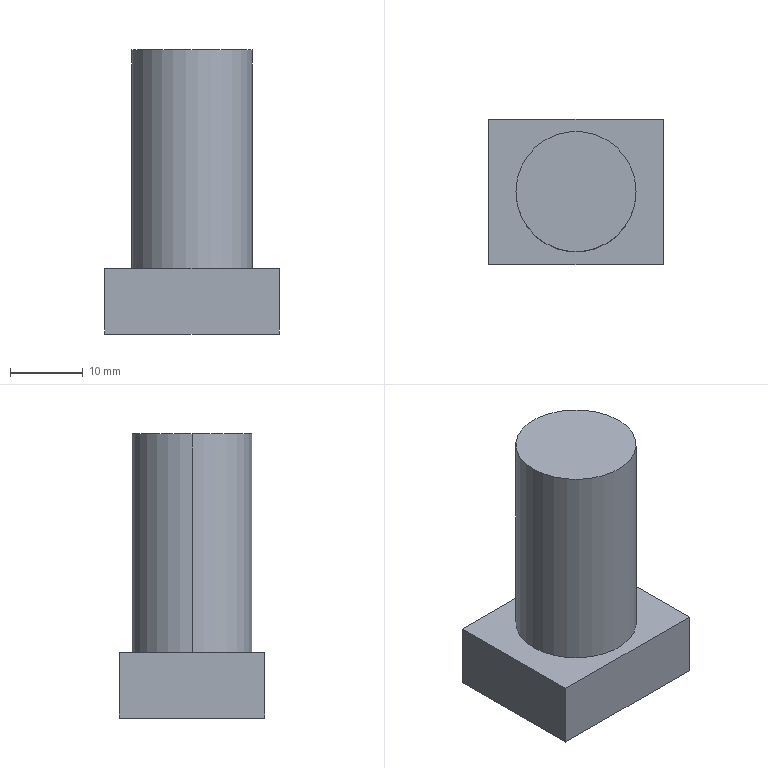Part | STEP file | Button | 1 solid | 9 faces | box 24 x 20 x 39 mm | volume 10735 mm3 | plane 7 | cylinder 2 | commonest cylinder face diameters 16.5 x2
STEP:
#1=CARTESIAN_POINT('',(0.,0.,0.));
#2=DIRECTION('',(0.,0.,1.));
#3=DIRECTION('',(1.,0.,0.));
#4=AXIS2_PLACEMENT_3D('',#1,#2,#3);
#5=CARTESIAN_POINT('',(-8.25,0.,39.));
#6=VERTEX_POINT('',#5);
#7=CARTESIAN_POINT('',(8.25,0.,39.));
#8=VERTEX_POINT('',#7);
#9=CARTESIAN_POINT('',(0.,0.,39.));
#10=DIRECTION('',(0.,0.,-1.));
#11=DIRECTION('',(-1.,0.,0.));
#12=AXIS2_PLACEMENT_3D('',#9,#10,#11);
#13=CIRCLE('',#12,8.25);
#14=CARTESIAN_POINT('',(0.,0.,39.));
#15=DIRECTION('',(0.,0.,-1.));
#16=DIRECTION('',(-1.,0.,0.));
#17=AXIS2_PLACEMENT_3D('',#14,#15,#16);
#18=CYLINDRICAL_SURFACE('',#17,8.25);
#19=CARTESIAN_POINT('',(0.,0.));
#20=DIRECTION('',(1.,0.));
#21=VECTOR('',#20,1.);
#22=LINE('',#19,#21);
#23=(GEOMETRIC_REPRESENTATION_CONTEXT(2)PARAMETRIC_REPRESENTATION_CONTEXT()REPRESENTATION_CONTEXT('',''));
#24=DEFINITIONAL_REPRESENTATION('',(#22),#23);
#25=PCURVE('',#18,#24);
#26=CARTESIAN_POINT('',(0.,0.,39.));
#27=DIRECTION('',(0.,0.,1.));
#28=DIRECTION('',(1.,0.,0.));
#29=AXIS2_PLACEMENT_3D('',#26,#27,#28);
#30=PLANE('',#29);
#31=CARTESIAN_POINT('',(-8.25,0.));
#32=CARTESIAN_POINT('',(-8.25,14.289));
#33=CARTESIAN_POINT('',(4.125,7.145));
#34=CARTESIAN_POINT('',(16.5,0.));
#35=CARTESIAN_POINT('',(4.125,-7.145));
#36=CARTESIAN_POINT('',(-8.25,-14.289));
#37=CARTESIAN_POINT('',(-8.25,0.));
#38=(BOUNDED_CURVE()B_SPLINE_CURVE(2,(#31,#32,#33,#34,#35,#36,#37),.UNSPECIFIED.,.T.,.F.)B_SPLINE_CURVE_WITH_KNOTS((1,2,2,2,2,1),(-2.094,0.,2.094,4.189,6.283,8.378),.UNSPECIFIED.)CURVE()GEOMETRIC_REPRESENTATION_ITEM()RATIONAL_B_SPLINE_CURVE((1.,0.5,1.,0.5,1.,0.5,1.))REPRESENTATION_ITEM(''));
#39=(GEOMETRIC_REPRESENTATION_CONTEXT(2)PARAMETRIC_REPRESENTATION_CONTEXT()REPRESENTATION_CONTEXT('',''));
#40=DEFINITIONAL_REPRESENTATION('',(#38),#39);
#41=PCURVE('',#30,#40);
#42=SURFACE_CURVE('',#13,(#25,#41),.PCURVE_S1.);
#43=EDGE_CURVE('',#6,#8,#42,.T.);
#44=ORIENTED_EDGE('',*,*,#43,.T.);
#45=CARTESIAN_POINT('',(8.25,0.,9.));
#46=VERTEX_POINT('',#45);
#47=CARTESIAN_POINT('',(8.25,0.,39.));
#48=DIRECTION('',(0.,0.,-1.));
#49=VECTOR('',#48,1.);
#50=LINE('',#47,#49);
#51=CARTESIAN_POINT('',(3.142,0.));
#52=DIRECTION('',(0.,1.));
#53=VECTOR('',#52,1.);
#54=LINE('',#51,#53);
#55=(GEOMETRIC_REPRESENTATION_CONTEXT(2)PARAMETRIC_REPRESENTATION_CONTEXT()REPRESENTATION_CONTEXT('',''));
#56=DEFINITIONAL_REPRESENTATION('',(#54),#55);
#57=PCURVE('',#18,#56);
#58=CARTESIAN_POINT('',(0.,0.,39.));
#59=DIRECTION('',(0.,0.,-1.));
#60=DIRECTION('',(-1.,0.,0.));
#61=AXIS2_PLACEMENT_3D('',#58,#59,#60);
#62=CYLINDRICAL_SURFACE('',#61,8.25);
#63=CARTESIAN_POINT('',(3.142,0.));
#64=DIRECTION('',(0.,1.));
#65=VECTOR('',#64,1.);
#66=LINE('',#63,#65);
#67=(GEOMETRIC_REPRESENTATION_CONTEXT(2)PARAMETRIC_REPRESENTATION_CONTEXT()REPRESENTATION_CONTEXT('',''));
#68=DEFINITIONAL_REPRESENTATION('',(#66),#67);
#69=PCURVE('',#62,#68);
#70=SURFACE_CURVE('',#50,(#57,#69),.PCURVE_S1.);
#71=EDGE_CURVE('',#8,#46,#70,.T.);
#72=ORIENTED_EDGE('',*,*,#71,.T.);
#73=CARTESIAN_POINT('',(-8.25,0.,9.));
#74=VERTEX_POINT('',#73);
#75=CARTESIAN_POINT('',(0.,0.,9.));
#76=DIRECTION('',(0.,0.,1.));
#77=DIRECTION('',(-1.,0.,0.));
#78=AXIS2_PLACEMENT_3D('',#75,#76,#77);
#79=CIRCLE('',#78,8.25);
#80=CARTESIAN_POINT('',(6.283,30.));
#81=DIRECTION('',(-1.,0.));
#82=VECTOR('',#81,1.);
#83=LINE('',#80,#82);
#84=(GEOMETRIC_REPRESENTATION_CONTEXT(2)PARAMETRIC_REPRESENTATION_CONTEXT()REPRESENTATION_CONTEXT('',''));
#85=DEFINITIONAL_REPRESENTATION('',(#83),#84);
#86=PCURVE('',#18,#85);
#87=CARTESIAN_POINT('',(-12.,-10.,9.));
#88=DIRECTION('',(0.,0.,1.));
#89=DIRECTION('',(1.,0.,0.));
#90=AXIS2_PLACEMENT_3D('',#87,#88,#89);
#91=PLANE('',#90);
#92=CARTESIAN_POINT('',(12.,10.));
#93=DIRECTION('',(-1.,0.));
#94=AXIS2_PLACEMENT_2D('',#92,#93);
#95=CIRCLE('',#94,8.25);
#96=(GEOMETRIC_REPRESENTATION_CONTEXT(2)PARAMETRIC_REPRESENTATION_CONTEXT()REPRESENTATION_CONTEXT('',''));
#97=DEFINITIONAL_REPRESENTATION('',(#95),#96);
#98=PCURVE('',#91,#97);
#99=SURFACE_CURVE('',#79,(#86,#98),.PCURVE_S1.);
#100=EDGE_CURVE('',#46,#74,#99,.T.);
#101=ORIENTED_EDGE('',*,*,#100,.T.);
#102=CARTESIAN_POINT('',(-8.25,0.,39.));
#103=DIRECTION('',(0.,0.,-1.));
#104=VECTOR('',#103,1.);
#105=LINE('',#102,#104);
#106=CARTESIAN_POINT('',(0.,0.));
#107=DIRECTION('',(0.,1.));
#108=VECTOR('',#107,1.);
#109=LINE('',#106,#108);
#110=(GEOMETRIC_REPRESENTATION_CONTEXT(2)PARAMETRIC_REPRESENTATION_CONTEXT()REPRESENTATION_CONTEXT('',''));
#111=DEFINITIONAL_REPRESENTATION('',(#109),#110);
#112=PCURVE('',#18,#111);
#113=CARTESIAN_POINT('',(6.283,0.));
#114=DIRECTION('',(0.,1.));
#115=VECTOR('',#114,1.);
#116=LINE('',#113,#115);
#117=(GEOMETRIC_REPRESENTATION_CONTEXT(2)PARAMETRIC_REPRESENTATION_CONTEXT()REPRESENTATION_CONTEXT('',''));
#118=DEFINITIONAL_REPRESENTATION('',(#116),#117);
#119=PCURVE('',#62,#118);
#120=SURFACE_CURVE('',#105,(#112,#119),.PCURVE_S1.);
#121=EDGE_CURVE('',#6,#74,#120,.T.);
#122=ORIENTED_EDGE('',*,*,#121,.F.);
#123=EDGE_LOOP('',(#44,#72,#101,#122));
#124=FACE_BOUND('',#123,.T.);
#125=ADVANCED_FACE('',(#124),#18,.T.);
#126=ORIENTED_EDGE('',*,*,#71,.F.);
#127=CARTESIAN_POINT('',(0.,0.,39.));
#128=DIRECTION('',(0.,0.,-1.));
#129=DIRECTION('',(-1.,0.,0.));
#130=AXIS2_PLACEMENT_3D('',#127,#128,#129);
#131=CIRCLE('',#130,8.25);
#132=CARTESIAN_POINT('',(0.,0.));
#133=DIRECTION('',(1.,0.));
#134=VECTOR('',#133,1.);
#135=LINE('',#132,#134);
#136=(GEOMETRIC_REPRESENTATION_CONTEXT(2)PARAMETRIC_REPRESENTATION_CONTEXT()REPRESENTATION_CONTEXT('',''));
#137=DEFINITIONAL_REPRESENTATION('',(#135),#136);
#138=PCURVE('',#62,#137);
#139=CARTESIAN_POINT('',(-8.25,0.));
#140=CARTESIAN_POINT('',(-8.25,14.289));
#141=CARTESIAN_POINT('',(4.125,7.145));
#142=CARTESIAN_POINT('',(16.5,0.));
#143=CARTESIAN_POINT('',(4.125,-7.145));
#144=CARTESIAN_POINT('',(-8.25,-14.289));
#145=CARTESIAN_POINT('',(-8.25,0.));
#146=(BOUNDED_CURVE()B_SPLINE_CURVE(2,(#139,#140,#141,#142,#143,#144,#145),.UNSPECIFIED.,.T.,.F.)B_SPLINE_CURVE_WITH_KNOTS((1,2,2,2,2,1),(-2.094,0.,2.094,4.189,6.283,8.378),.UNSPECIFIED.)CURVE()GEOMETRIC_REPRESENTATION_ITEM()RATIONAL_B_SPLINE_CURVE((1.,0.5,1.,0.5,1.,0.5,1.))REPRESENTATION_ITEM(''));
#147=(GEOMETRIC_REPRESENTATION_CONTEXT(2)PARAMETRIC_REPRESENTATION_CONTEXT()REPRESENTATION_CONTEXT('',''));
#148=DEFINITIONAL_REPRESENTATION('',(#146),#147);
#149=PCURVE('',#30,#148);
#150=SURFACE_CURVE('',#131,(#138,#149),.PCURVE_S1.);
#151=EDGE_CURVE('',#8,#6,#150,.T.);
#152=ORIENTED_EDGE('',*,*,#151,.T.);
#153=ORIENTED_EDGE('',*,*,#121,.T.);
#154=CARTESIAN_POINT('',(0.,0.,9.));
#155=DIRECTION('',(0.,0.,1.));
#156=DIRECTION('',(-1.,0.,0.));
#157=AXIS2_PLACEMENT_3D('',#154,#155,#156);
#158=CIRCLE('',#157,8.25);
#159=CARTESIAN_POINT('',(6.283,30.));
#160=DIRECTION('',(-1.,0.));
#161=VECTOR('',#160,1.);
#162=LINE('',#159,#161);
#163=(GEOMETRIC_REPRESENTATION_CONTEXT(2)PARAMETRIC_REPRESENTATION_CONTEXT()REPRESENTATION_CONTEXT('',''));
#164=DEFINITIONAL_REPRESENTATION('',(#162),#163);
#165=PCURVE('',#62,#164);
#166=CARTESIAN_POINT('',(12.,10.));
#167=DIRECTION('',(-1.,0.));
#168=AXIS2_PLACEMENT_2D('',#166,#167);
#169=CIRCLE('',#168,8.25);
#170=(GEOMETRIC_REPRESENTATION_CONTEXT(2)PARAMETRIC_REPRESENTATION_CONTEXT()REPRESENTATION_CONTEXT('',''));
#171=DEFINITIONAL_REPRESENTATION('',(#169),#170);
#172=PCURVE('',#91,#171);
#173=SURFACE_CURVE('',#158,(#165,#172),.PCURVE_S1.);
#174=EDGE_CURVE('',#74,#46,#173,.T.);
#175=ORIENTED_EDGE('',*,*,#174,.T.);
#176=EDGE_LOOP('',(#126,#152,#153,#175));
#177=FACE_BOUND('',#176,.T.);
#178=ADVANCED_FACE('',(#177),#62,.T.);
#179=ORIENTED_EDGE('',*,*,#174,.F.);
#180=ORIENTED_EDGE('',*,*,#100,.F.);
#181=EDGE_LOOP('',(#179,#180));
#182=FACE_BOUND('',#181,.T.);
#183=CARTESIAN_POINT('',(12.,-10.,9.));
#184=VERTEX_POINT('',#183);
#185=CARTESIAN_POINT('',(12.,10.,9.));
#186=VERTEX_POINT('',#185);
#187=CARTESIAN_POINT('',(12.,-10.,9.));
#188=DIRECTION('',(0.,1.,0.));
#189=VECTOR('',#188,1.);
#190=LINE('',#187,#189);
#191=CARTESIAN_POINT('',(24.,0.));
#192=DIRECTION('',(0.,1.));
#193=VECTOR('',#192,1.);
#194=LINE('',#191,#193);
#195=(GEOMETRIC_REPRESENTATION_CONTEXT(2)PARAMETRIC_REPRESENTATION_CONTEXT()REPRESENTATION_CONTEXT('',''));
#196=DEFINITIONAL_REPRESENTATION('',(#194),#195);
#197=PCURVE('',#91,#196);
#198=CARTESIAN_POINT('',(12.,10.,9.));
#199=DIRECTION('',(-1.,0.,0.));
#200=DIRECTION('',(0.,0.,1.));
#201=AXIS2_PLACEMENT_3D('',#198,#199,#200);
#202=PLANE('',#201);
#203=CARTESIAN_POINT('',(0.,-20.));
#204=DIRECTION('',(0.,1.));
#205=VECTOR('',#204,1.);
#206=LINE('',#203,#205);
#207=(GEOMETRIC_REPRESENTATION_CONTEXT(2)PARAMETRIC_REPRESENTATION_CONTEXT()REPRESENTATION_CONTEXT('',''));
#208=DEFINITIONAL_REPRESENTATION('',(#206),#207);
#209=PCURVE('',#202,#208);
#210=SURFACE_CURVE('',#190,(#197,#209),.PCURVE_S1.);
#211=EDGE_CURVE('',#184,#186,#210,.T.);
#212=ORIENTED_EDGE('',*,*,#211,.T.);
#213=CARTESIAN_POINT('',(-12.,10.,9.));
#214=VERTEX_POINT('',#213);
#215=CARTESIAN_POINT('',(-12.,10.,9.));
#216=DIRECTION('',(-1.,0.,0.));
#217=VECTOR('',#216,1.);
#218=LINE('',#215,#217);
#219=CARTESIAN_POINT('',(0.,20.));
#220=DIRECTION('',(-1.,0.));
#221=VECTOR('',#220,1.);
#222=LINE('',#219,#221);
#223=(GEOMETRIC_REPRESENTATION_CONTEXT(2)PARAMETRIC_REPRESENTATION_CONTEXT()REPRESENTATION_CONTEXT('',''));
#224=DEFINITIONAL_REPRESENTATION('',(#222),#223);
#225=PCURVE('',#91,#224);
#226=CARTESIAN_POINT('',(-12.,10.,9.));
#227=DIRECTION('',(0.,-1.,0.));
#228=DIRECTION('',(0.,0.,-1.));
#229=AXIS2_PLACEMENT_3D('',#226,#227,#228);
#230=PLANE('',#229);
#231=CARTESIAN_POINT('',(0.,0.));
#232=DIRECTION('',(0.,-1.));
#233=VECTOR('',#232,1.);
#234=LINE('',#231,#233);
#235=(GEOMETRIC_REPRESENTATION_CONTEXT(2)PARAMETRIC_REPRESENTATION_CONTEXT()REPRESENTATION_CONTEXT('',''));
#236=DEFINITIONAL_REPRESENTATION('',(#234),#235);
#237=PCURVE('',#230,#236);
#238=SURFACE_CURVE('',#218,(#225,#237),.PCURVE_S1.);
#239=EDGE_CURVE('',#186,#214,#238,.T.);
#240=ORIENTED_EDGE('',*,*,#239,.T.);
#241=CARTESIAN_POINT('',(-12.,-10.,9.));
#242=VERTEX_POINT('',#241);
#243=CARTESIAN_POINT('',(-12.,-10.,9.));
#244=DIRECTION('',(0.,-1.,0.));
#245=VECTOR('',#244,1.);
#246=LINE('',#243,#245);
#247=CARTESIAN_POINT('',(0.,0.));
#248=DIRECTION('',(0.,-1.));
#249=VECTOR('',#248,1.);
#250=LINE('',#247,#249);
#251=(GEOMETRIC_REPRESENTATION_CONTEXT(2)PARAMETRIC_REPRESENTATION_CONTEXT()REPRESENTATION_CONTEXT('',''));
#252=DEFINITIONAL_REPRESENTATION('',(#250),#251);
#253=PCURVE('',#91,#252);
#254=CARTESIAN_POINT('',(-12.,10.,9.));
#255=DIRECTION('',(1.,0.,0.));
#256=DIRECTION('',(0.,0.,-1.));
#257=AXIS2_PLACEMENT_3D('',#254,#255,#256);
#258=PLANE('',#257);
#259=CARTESIAN_POINT('',(0.,-20.));
#260=DIRECTION('',(0.,-1.));
#261=VECTOR('',#260,1.);
#262=LINE('',#259,#261);
#263=(GEOMETRIC_REPRESENTATION_CONTEXT(2)PARAMETRIC_REPRESENTATION_CONTEXT()REPRESENTATION_CONTEXT('',''));
#264=DEFINITIONAL_REPRESENTATION('',(#262),#263);
#265=PCURVE('',#258,#264);
#266=SURFACE_CURVE('',#246,(#253,#265),.PCURVE_S1.);
#267=EDGE_CURVE('',#214,#242,#266,.T.);
#268=ORIENTED_EDGE('',*,*,#267,.T.);
#269=CARTESIAN_POINT('',(-12.,-10.,9.));
#270=DIRECTION('',(1.,0.,0.));
#271=VECTOR('',#270,1.);
#272=LINE('',#269,#271);
#273=CARTESIAN_POINT('',(0.,0.));
#274=DIRECTION('',(1.,0.));
#275=VECTOR('',#274,1.);
#276=LINE('',#273,#275);
#277=(GEOMETRIC_REPRESENTATION_CONTEXT(2)PARAMETRIC_REPRESENTATION_CONTEXT()REPRESENTATION_CONTEXT('',''));
#278=DEFINITIONAL_REPRESENTATION('',(#276),#277);
#279=PCURVE('',#91,#278);
#280=CARTESIAN_POINT('',(-12.,-10.,9.));
#281=DIRECTION('',(0.,1.,0.));
#282=DIRECTION('',(0.,0.,1.));
#283=AXIS2_PLACEMENT_3D('',#280,#281,#282);
#284=PLANE('',#283);
#285=CARTESIAN_POINT('',(0.,0.));
#286=DIRECTION('',(0.,1.));
#287=VECTOR('',#286,1.);
#288=LINE('',#285,#287);
#289=(GEOMETRIC_REPRESENTATION_CONTEXT(2)PARAMETRIC_REPRESENTATION_CONTEXT()REPRESENTATION_CONTEXT('',''));
#290=DEFINITIONAL_REPRESENTATION('',(#288),#289);
#291=PCURVE('',#284,#290);
#292=SURFACE_CURVE('',#272,(#279,#291),.PCURVE_S1.);
#293=EDGE_CURVE('',#242,#184,#292,.T.);
#294=ORIENTED_EDGE('',*,*,#293,.T.);
#295=EDGE_LOOP('',(#212,#240,#268,#294));
#296=FACE_BOUND('',#295,.T.);
#297=ADVANCED_FACE('',(#182,#296),#91,.T.);
#298=ORIENTED_EDGE('',*,*,#43,.F.);
#299=ORIENTED_EDGE('',*,*,#151,.F.);
#300=EDGE_LOOP('',(#298,#299));
#301=FACE_BOUND('',#300,.T.);
#302=ADVANCED_FACE('',(#301),#30,.T.);
#303=CARTESIAN_POINT('',(-12.,10.,0.));
#304=VERTEX_POINT('',#303);
#305=CARTESIAN_POINT('',(-12.,10.,9.));
#306=DIRECTION('',(0.,0.,-1.));
#307=VECTOR('',#306,1.);
#308=LINE('',#305,#307);
#309=CARTESIAN_POINT('',(0.,0.));
#310=DIRECTION('',(1.,0.));
#311=VECTOR('',#310,1.);
#312=LINE('',#309,#311);
#313=(GEOMETRIC_REPRESENTATION_CONTEXT(2)PARAMETRIC_REPRESENTATION_CONTEXT()REPRESENTATION_CONTEXT('',''));
#314=DEFINITIONAL_REPRESENTATION('',(#312),#313);
#315=PCURVE('',#230,#314);
#316=CARTESIAN_POINT('',(0.,0.));
#317=DIRECTION('',(1.,0.));
#318=VECTOR('',#317,1.);
#319=LINE('',#316,#318);
#320=(GEOMETRIC_REPRESENTATION_CONTEXT(2)PARAMETRIC_REPRESENTATION_CONTEXT()REPRESENTATION_CONTEXT('',''));
#321=DEFINITIONAL_REPRESENTATION('',(#319),#320);
#322=PCURVE('',#258,#321);
#323=SURFACE_CURVE('',#308,(#315,#322),.PCURVE_S1.);
#324=EDGE_CURVE('',#214,#304,#323,.T.);
#325=ORIENTED_EDGE('',*,*,#324,.F.);
#326=ORIENTED_EDGE('',*,*,#239,.F.);
#327=CARTESIAN_POINT('',(12.,10.,0.));
#328=VERTEX_POINT('',#327);
#329=CARTESIAN_POINT('',(12.,10.,9.));
#330=DIRECTION('',(0.,0.,1.));
#331=VECTOR('',#330,1.);
#332=LINE('',#329,#331);
#333=CARTESIAN_POINT('',(0.,24.));
#334=DIRECTION('',(-1.,0.));
#335=VECTOR('',#334,1.);
#336=LINE('',#333,#335);
#337=(GEOMETRIC_REPRESENTATION_CONTEXT(2)PARAMETRIC_REPRESENTATION_CONTEXT()REPRESENTATION_CONTEXT('',''));
#338=DEFINITIONAL_REPRESENTATION('',(#336),#337);
#339=PCURVE('',#230,#338);
#340=CARTESIAN_POINT('',(0.,0.));
#341=DIRECTION('',(1.,0.));
#342=VECTOR('',#341,1.);
#343=LINE('',#340,#342);
#344=(GEOMETRIC_REPRESENTATION_CONTEXT(2)PARAMETRIC_REPRESENTATION_CONTEXT()REPRESENTATION_CONTEXT('',''));
#345=DEFINITIONAL_REPRESENTATION('',(#343),#344);
#346=PCURVE('',#202,#345);
#347=SURFACE_CURVE('',#332,(#339,#346),.PCURVE_S1.);
#348=EDGE_CURVE('',#328,#186,#347,.T.);
#349=ORIENTED_EDGE('',*,*,#348,.F.);
#350=CARTESIAN_POINT('',(-12.,10.,0.));
#351=DIRECTION('',(1.,0.,0.));
#352=VECTOR('',#351,1.);
#353=LINE('',#350,#352);
#354=CARTESIAN_POINT('',(9.,0.));
#355=DIRECTION('',(0.,1.));
#356=VECTOR('',#355,1.);
#357=LINE('',#354,#356);
#358=(GEOMETRIC_REPRESENTATION_CONTEXT(2)PARAMETRIC_REPRESENTATION_CONTEXT()REPRESENTATION_CONTEXT('',''));
#359=DEFINITIONAL_REPRESENTATION('',(#357),#358);
#360=PCURVE('',#230,#359);
#361=CARTESIAN_POINT('',(-12.,-10.,0.));
#362=DIRECTION('',(0.,0.,1.));
#363=DIRECTION('',(1.,0.,0.));
#364=AXIS2_PLACEMENT_3D('',#361,#362,#363);
#365=PLANE('',#364);
#366=CARTESIAN_POINT('',(0.,20.));
#367=DIRECTION('',(1.,0.));
#368=VECTOR('',#367,1.);
#369=LINE('',#366,#368);
#370=(GEOMETRIC_REPRESENTATION_CONTEXT(2)PARAMETRIC_REPRESENTATION_CONTEXT()REPRESENTATION_CONTEXT('',''));
#371=DEFINITIONAL_REPRESENTATION('',(#369),#370);
#372=PCURVE('',#365,#371);
#373=SURFACE_CURVE('',#353,(#360,#372),.PCURVE_S1.);
#374=EDGE_CURVE('',#304,#328,#373,.T.);
#375=ORIENTED_EDGE('',*,*,#374,.F.);
#376=EDGE_LOOP('',(#325,#326,#349,#375));
#377=FACE_BOUND('',#376,.T.);
#378=ADVANCED_FACE('',(#377),#230,.F.);
#379=ORIENTED_EDGE('',*,*,#348,.T.);
#380=ORIENTED_EDGE('',*,*,#211,.F.);
#381=CARTESIAN_POINT('',(12.,-10.,0.));
#382=VERTEX_POINT('',#381);
#383=CARTESIAN_POINT('',(12.,-10.,9.));
#384=DIRECTION('',(0.,0.,1.));
#385=VECTOR('',#384,1.);
#386=LINE('',#383,#385);
#387=CARTESIAN_POINT('',(0.,-20.));
#388=DIRECTION('',(1.,0.));
#389=VECTOR('',#388,1.);
#390=LINE('',#387,#389);
#391=(GEOMETRIC_REPRESENTATION_CONTEXT(2)PARAMETRIC_REPRESENTATION_CONTEXT()REPRESENTATION_CONTEXT('',''));
#392=DEFINITIONAL_REPRESENTATION('',(#390),#391);
#393=PCURVE('',#202,#392);
#394=CARTESIAN_POINT('',(0.,24.));
#395=DIRECTION('',(1.,0.));
#396=VECTOR('',#395,1.);
#397=LINE('',#394,#396);
#398=(GEOMETRIC_REPRESENTATION_CONTEXT(2)PARAMETRIC_REPRESENTATION_CONTEXT()REPRESENTATION_CONTEXT('',''));
#399=DEFINITIONAL_REPRESENTATION('',(#397),#398);
#400=PCURVE('',#284,#399);
#401=SURFACE_CURVE('',#386,(#393,#400),.PCURVE_S1.);
#402=EDGE_CURVE('',#382,#184,#401,.T.);
#403=ORIENTED_EDGE('',*,*,#402,.F.);
#404=CARTESIAN_POINT('',(12.,10.,0.));
#405=DIRECTION('',(0.,-1.,0.));
#406=VECTOR('',#405,1.);
#407=LINE('',#404,#406);
#408=CARTESIAN_POINT('',(-9.,0.));
#409=DIRECTION('',(0.,-1.));
#410=VECTOR('',#409,1.);
#411=LINE('',#408,#410);
#412=(GEOMETRIC_REPRESENTATION_CONTEXT(2)PARAMETRIC_REPRESENTATION_CONTEXT()REPRESENTATION_CONTEXT('',''));
#413=DEFINITIONAL_REPRESENTATION('',(#411),#412);
#414=PCURVE('',#202,#413);
#415=CARTESIAN_POINT('',(24.,20.));
#416=DIRECTION('',(0.,-1.));
#417=VECTOR('',#416,1.);
#418=LINE('',#415,#417);
#419=(GEOMETRIC_REPRESENTATION_CONTEXT(2)PARAMETRIC_REPRESENTATION_CONTEXT()REPRESENTATION_CONTEXT('',''));
#420=DEFINITIONAL_REPRESENTATION('',(#418),#419);
#421=PCURVE('',#365,#420);
#422=SURFACE_CURVE('',#407,(#414,#421),.PCURVE_S1.);
#423=EDGE_CURVE('',#328,#382,#422,.T.);
#424=ORIENTED_EDGE('',*,*,#423,.F.);
#425=EDGE_LOOP('',(#379,#380,#403,#424));
#426=FACE_BOUND('',#425,.T.);
#427=ADVANCED_FACE('',(#426),#202,.F.);
#428=ORIENTED_EDGE('',*,*,#402,.T.);
#429=ORIENTED_EDGE('',*,*,#293,.F.);
#430=CARTESIAN_POINT('',(-12.,-10.,0.));
#431=VERTEX_POINT('',#430);
#432=CARTESIAN_POINT('',(-12.,-10.,9.));
#433=DIRECTION('',(0.,0.,1.));
#434=VECTOR('',#433,1.);
#435=LINE('',#432,#434);
#436=CARTESIAN_POINT('',(0.,0.));
#437=DIRECTION('',(1.,0.));
#438=VECTOR('',#437,1.);
#439=LINE('',#436,#438);
#440=(GEOMETRIC_REPRESENTATION_CONTEXT(2)PARAMETRIC_REPRESENTATION_CONTEXT()REPRESENTATION_CONTEXT('',''));
#441=DEFINITIONAL_REPRESENTATION('',(#439),#440);
#442=PCURVE('',#284,#441);
#443=CARTESIAN_POINT('',(0.,-20.));
#444=DIRECTION('',(-1.,0.));
#445=VECTOR('',#444,1.);
#446=LINE('',#443,#445);
#447=(GEOMETRIC_REPRESENTATION_CONTEXT(2)PARAMETRIC_REPRESENTATION_CONTEXT()REPRESENTATION_CONTEXT('',''));
#448=DEFINITIONAL_REPRESENTATION('',(#446),#447);
#449=PCURVE('',#258,#448);
#450=SURFACE_CURVE('',#435,(#442,#449),.PCURVE_S1.);
#451=EDGE_CURVE('',#431,#242,#450,.T.);
#452=ORIENTED_EDGE('',*,*,#451,.F.);
#453=CARTESIAN_POINT('',(-12.,-10.,0.));
#454=DIRECTION('',(-1.,0.,0.));
#455=VECTOR('',#454,1.);
#456=LINE('',#453,#455);
#457=CARTESIAN_POINT('',(-9.,0.));
#458=DIRECTION('',(0.,-1.));
#459=VECTOR('',#458,1.);
#460=LINE('',#457,#459);
#461=(GEOMETRIC_REPRESENTATION_CONTEXT(2)PARAMETRIC_REPRESENTATION_CONTEXT()REPRESENTATION_CONTEXT('',''));
#462=DEFINITIONAL_REPRESENTATION('',(#460),#461);
#463=PCURVE('',#284,#462);
#464=CARTESIAN_POINT('',(0.,0.));
#465=DIRECTION('',(-1.,0.));
#466=VECTOR('',#465,1.);
#467=LINE('',#464,#466);
#468=(GEOMETRIC_REPRESENTATION_CONTEXT(2)PARAMETRIC_REPRESENTATION_CONTEXT()REPRESENTATION_CONTEXT('',''));
#469=DEFINITIONAL_REPRESENTATION('',(#467),#468);
#470=PCURVE('',#365,#469);
#471=SURFACE_CURVE('',#456,(#463,#470),.PCURVE_S1.);
#472=EDGE_CURVE('',#382,#431,#471,.T.);
#473=ORIENTED_EDGE('',*,*,#472,.F.);
#474=EDGE_LOOP('',(#428,#429,#452,#473));
#475=FACE_BOUND('',#474,.T.);
#476=ADVANCED_FACE('',(#475),#284,.F.);
#477=ORIENTED_EDGE('',*,*,#451,.T.);
#478=ORIENTED_EDGE('',*,*,#267,.F.);
#479=ORIENTED_EDGE('',*,*,#324,.T.);
#480=CARTESIAN_POINT('',(-12.,10.,0.));
#481=DIRECTION('',(0.,1.,0.));
#482=VECTOR('',#481,1.);
#483=LINE('',#480,#482);
#484=CARTESIAN_POINT('',(9.,0.));
#485=DIRECTION('',(0.,1.));
#486=VECTOR('',#485,1.);
#487=LINE('',#484,#486);
#488=(GEOMETRIC_REPRESENTATION_CONTEXT(2)PARAMETRIC_REPRESENTATION_CONTEXT()REPRESENTATION_CONTEXT('',''));
#489=DEFINITIONAL_REPRESENTATION('',(#487),#488);
#490=PCURVE('',#258,#489);
#491=CARTESIAN_POINT('',(0.,20.));
#492=DIRECTION('',(0.,1.));
#493=VECTOR('',#492,1.);
#494=LINE('',#491,#493);
#495=(GEOMETRIC_REPRESENTATION_CONTEXT(2)PARAMETRIC_REPRESENTATION_CONTEXT()REPRESENTATION_CONTEXT('',''));
#496=DEFINITIONAL_REPRESENTATION('',(#494),#495);
#497=PCURVE('',#365,#496);
#498=SURFACE_CURVE('',#483,(#490,#497),.PCURVE_S1.);
#499=EDGE_CURVE('',#431,#304,#498,.T.);
#500=ORIENTED_EDGE('',*,*,#499,.F.);
#501=EDGE_LOOP('',(#477,#478,#479,#500));
#502=FACE_BOUND('',#501,.T.);
#503=ADVANCED_FACE('',(#502),#258,.F.);
#504=ORIENTED_EDGE('',*,*,#374,.T.);
#505=ORIENTED_EDGE('',*,*,#423,.T.);
#506=ORIENTED_EDGE('',*,*,#472,.T.);
#507=ORIENTED_EDGE('',*,*,#499,.T.);
#508=EDGE_LOOP('',(#504,#505,#506,#507));
#509=FACE_BOUND('',#508,.T.);
#510=ADVANCED_FACE('',(#509),#365,.F.);
#511=CLOSED_SHELL('',(#125,#178,#297,#302,#378,#427,#476,#503,#510));
#512=MANIFOLD_SOLID_BREP('',#511);
#513=(LENGTH_UNIT()NAMED_UNIT(*)SI_UNIT(.MILLI.,.METRE.));
#514=UNCERTAINTY_MEASURE_WITH_UNIT(LENGTH_MEASURE(0.0000001),#513,'','');
#515=(NAMED_UNIT(*)PLANE_ANGLE_UNIT()SI_UNIT($,.RADIAN.));
#516=(NAMED_UNIT(*)SI_UNIT($,.STERADIAN.)SOLID_ANGLE_UNIT());
#517=(GEOMETRIC_REPRESENTATION_CONTEXT(3)GLOBAL_UNCERTAINTY_ASSIGNED_CONTEXT((#514))GLOBAL_UNIT_ASSIGNED_CONTEXT((#513,#515,#516))REPRESENTATION_CONTEXT('',''));
#518=ADVANCED_BREP_SHAPE_REPRESENTATION('',(#4,#512),#517);